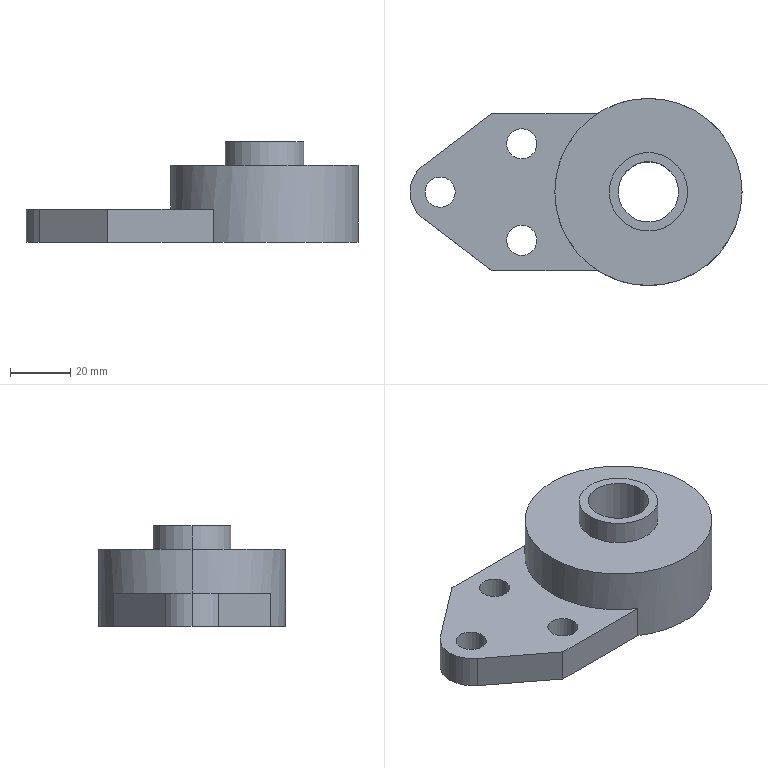Part | SolidWorks | features ICE 2, Extrusion 1 | 1 solid | 22 faces | box 110 x 62 x 33.3 mm | volume 91720 mm3 | cylinder 14 | plane 8 | commonest cylinder face diameters 10 x6 20 x2 22 x2 26 x2 62 x2
STEP:
#1=CARTESIAN_POINT('',(13.,0.,33.3));
#2=VERTEX_POINT('',#1);
#3=CARTESIAN_POINT('',(-13.,0.,33.3));
#4=VERTEX_POINT('',#3);
#5=CARTESIAN_POINT('',(0.,0.,33.3));
#6=DIRECTION('',(0.,0.,1.));
#7=DIRECTION('',(1.,0.,0.));
#8=AXIS2_PLACEMENT_3D('',#5,#6,#7);
#9=CIRCLE('',#8,13.);
#10=EDGE_CURVE('',#2,#4,#9,.T.);
#11=ORIENTED_EDGE('',*,*,#10,.F.);
#12=CARTESIAN_POINT('',(13.,0.,25.5));
#13=VERTEX_POINT('',#12);
#14=CARTESIAN_POINT('',(13.,0.,33.3));
#15=DIRECTION('',(0.,0.,-1.));
#16=VECTOR('',#15,1000.);
#17=LINE('',#14,#16);
#18=EDGE_CURVE('',#2,#13,#17,.T.);
#19=ORIENTED_EDGE('',*,*,#18,.T.);
#20=CARTESIAN_POINT('',(-13.,0.,25.5));
#21=VERTEX_POINT('',#20);
#22=CARTESIAN_POINT('',(0.,0.,25.5));
#23=DIRECTION('',(0.,0.,1.));
#24=DIRECTION('',(1.,0.,0.));
#25=AXIS2_PLACEMENT_3D('',#22,#23,#24);
#26=CIRCLE('',#25,13.);
#27=EDGE_CURVE('',#13,#21,#26,.T.);
#28=ORIENTED_EDGE('',*,*,#27,.T.);
#29=CARTESIAN_POINT('',(-13.,0.,33.3));
#30=DIRECTION('',(0.,0.,-1.));
#31=VECTOR('',#30,1000.);
#32=LINE('',#29,#31);
#33=EDGE_CURVE('',#4,#21,#32,.T.);
#34=ORIENTED_EDGE('',*,*,#33,.F.);
#35=EDGE_LOOP('',(#11,#19,#28,#34));
#36=FACE_OUTER_BOUND('',#35,.T.);
#37=CARTESIAN_POINT('',(0.,0.,33.3));
#38=DIRECTION('',(0.,0.,-1.));
#39=DIRECTION('',(-1.,0.,0.));
#40=AXIS2_PLACEMENT_3D('',#37,#38,#39);
#41=CYLINDRICAL_SURFACE('',#40,13.);
#42=ADVANCED_FACE('',(#36),#41,.T.);
#43=CARTESIAN_POINT('',(-37.,-16.,11.));
#44=VERTEX_POINT('',#43);
#45=CARTESIAN_POINT('',(-47.,-16.,11.));
#46=VERTEX_POINT('',#45);
#47=CARTESIAN_POINT('',(-42.,-16.,11.));
#48=DIRECTION('',(0.,0.,-1.));
#49=DIRECTION('',(-1.,0.,0.));
#50=AXIS2_PLACEMENT_3D('',#47,#48,#49);
#51=CIRCLE('',#50,5.);
#52=EDGE_CURVE('',#44,#46,#51,.T.);
#53=ORIENTED_EDGE('',*,*,#52,.F.);
#54=CARTESIAN_POINT('',(-37.,-16.,0.));
#55=VERTEX_POINT('',#54);
#56=CARTESIAN_POINT('',(-37.,-16.,11.));
#57=DIRECTION('',(0.,0.,-1.));
#58=VECTOR('',#57,1000.);
#59=LINE('',#56,#58);
#60=EDGE_CURVE('',#44,#55,#59,.T.);
#61=ORIENTED_EDGE('',*,*,#60,.T.);
#62=CARTESIAN_POINT('',(-47.,-16.,0.));
#63=VERTEX_POINT('',#62);
#64=CARTESIAN_POINT('',(-42.,-16.,0.));
#65=DIRECTION('',(0.,0.,-1.));
#66=DIRECTION('',(-1.,0.,0.));
#67=AXIS2_PLACEMENT_3D('',#64,#65,#66);
#68=CIRCLE('',#67,5.);
#69=EDGE_CURVE('',#55,#63,#68,.T.);
#70=ORIENTED_EDGE('',*,*,#69,.T.);
#71=CARTESIAN_POINT('',(-47.,-16.,11.));
#72=DIRECTION('',(0.,0.,-1.));
#73=VECTOR('',#72,1000.);
#74=LINE('',#71,#73);
#75=EDGE_CURVE('',#46,#63,#74,.T.);
#76=ORIENTED_EDGE('',*,*,#75,.F.);
#77=EDGE_LOOP('',(#53,#61,#70,#76));
#78=FACE_OUTER_BOUND('',#77,.T.);
#79=CARTESIAN_POINT('',(-42.,-16.,11.));
#80=DIRECTION('',(0.,0.,-1.));
#81=DIRECTION('',(-1.,0.,0.));
#82=AXIS2_PLACEMENT_3D('',#79,#80,#81);
#83=CYLINDRICAL_SURFACE('',#82,5.);
#84=ADVANCED_FACE('',(#78),#83,.F.);
#85=CARTESIAN_POINT('',(-37.,16.,11.));
#86=VERTEX_POINT('',#85);
#87=CARTESIAN_POINT('',(-47.,16.,11.));
#88=VERTEX_POINT('',#87);
#89=CARTESIAN_POINT('',(-42.,16.,11.));
#90=DIRECTION('',(0.,0.,-1.));
#91=DIRECTION('',(-1.,0.,0.));
#92=AXIS2_PLACEMENT_3D('',#89,#90,#91);
#93=CIRCLE('',#92,5.);
#94=EDGE_CURVE('',#86,#88,#93,.T.);
#95=ORIENTED_EDGE('',*,*,#94,.F.);
#96=CARTESIAN_POINT('',(-37.,16.,0.));
#97=VERTEX_POINT('',#96);
#98=CARTESIAN_POINT('',(-37.,16.,11.));
#99=DIRECTION('',(0.,0.,-1.));
#100=VECTOR('',#99,1000.);
#101=LINE('',#98,#100);
#102=EDGE_CURVE('',#86,#97,#101,.T.);
#103=ORIENTED_EDGE('',*,*,#102,.T.);
#104=CARTESIAN_POINT('',(-47.,16.,0.));
#105=VERTEX_POINT('',#104);
#106=CARTESIAN_POINT('',(-42.,16.,0.));
#107=DIRECTION('',(0.,0.,-1.));
#108=DIRECTION('',(-1.,0.,0.));
#109=AXIS2_PLACEMENT_3D('',#106,#107,#108);
#110=CIRCLE('',#109,5.);
#111=EDGE_CURVE('',#97,#105,#110,.T.);
#112=ORIENTED_EDGE('',*,*,#111,.T.);
#113=CARTESIAN_POINT('',(-47.,16.,11.));
#114=DIRECTION('',(0.,0.,-1.));
#115=VECTOR('',#114,1000.);
#116=LINE('',#113,#115);
#117=EDGE_CURVE('',#88,#105,#116,.T.);
#118=ORIENTED_EDGE('',*,*,#117,.F.);
#119=EDGE_LOOP('',(#95,#103,#112,#118));
#120=FACE_OUTER_BOUND('',#119,.T.);
#121=CARTESIAN_POINT('',(-42.,16.,11.));
#122=DIRECTION('',(0.,0.,-1.));
#123=DIRECTION('',(-1.,0.,0.));
#124=AXIS2_PLACEMENT_3D('',#121,#122,#123);
#125=CYLINDRICAL_SURFACE('',#124,5.);
#126=ADVANCED_FACE('',(#120),#125,.F.);
#127=CARTESIAN_POINT('',(-64.,0.,11.));
#128=VERTEX_POINT('',#127);
#129=CARTESIAN_POINT('',(-74.,0.,11.));
#130=VERTEX_POINT('',#129);
#131=CARTESIAN_POINT('',(-69.,0.,11.));
#132=DIRECTION('',(0.,0.,-1.));
#133=DIRECTION('',(-1.,0.,0.));
#134=AXIS2_PLACEMENT_3D('',#131,#132,#133);
#135=CIRCLE('',#134,5.);
#136=EDGE_CURVE('',#128,#130,#135,.T.);
#137=ORIENTED_EDGE('',*,*,#136,.F.);
#138=CARTESIAN_POINT('',(-64.,0.,0.));
#139=VERTEX_POINT('',#138);
#140=CARTESIAN_POINT('',(-64.,0.,11.));
#141=DIRECTION('',(0.,0.,-1.));
#142=VECTOR('',#141,1000.);
#143=LINE('',#140,#142);
#144=EDGE_CURVE('',#128,#139,#143,.T.);
#145=ORIENTED_EDGE('',*,*,#144,.T.);
#146=CARTESIAN_POINT('',(-74.,0.,0.));
#147=VERTEX_POINT('',#146);
#148=CARTESIAN_POINT('',(-69.,0.,0.));
#149=DIRECTION('',(0.,0.,-1.));
#150=DIRECTION('',(-1.,0.,0.));
#151=AXIS2_PLACEMENT_3D('',#148,#149,#150);
#152=CIRCLE('',#151,5.);
#153=EDGE_CURVE('',#139,#147,#152,.T.);
#154=ORIENTED_EDGE('',*,*,#153,.T.);
#155=CARTESIAN_POINT('',(-74.,0.,11.));
#156=DIRECTION('',(0.,0.,-1.));
#157=VECTOR('',#156,1000.);
#158=LINE('',#155,#157);
#159=EDGE_CURVE('',#130,#147,#158,.T.);
#160=ORIENTED_EDGE('',*,*,#159,.F.);
#161=EDGE_LOOP('',(#137,#145,#154,#160));
#162=FACE_OUTER_BOUND('',#161,.T.);
#163=CARTESIAN_POINT('',(-69.,0.,11.));
#164=DIRECTION('',(0.,0.,-1.));
#165=DIRECTION('',(-1.,0.,0.));
#166=AXIS2_PLACEMENT_3D('',#163,#164,#165);
#167=CYLINDRICAL_SURFACE('',#166,5.);
#168=ADVANCED_FACE('',(#162),#167,.F.);
#169=CARTESIAN_POINT('',(-74.662,-8.753,11.));
#170=VERTEX_POINT('',#169);
#171=CARTESIAN_POINT('',(-79.,0.,11.));
#172=VERTEX_POINT('',#171);
#173=CARTESIAN_POINT('',(-68.,0.,11.));
#174=DIRECTION('',(0.,0.,-1.));
#175=DIRECTION('',(-1.,0.,0.));
#176=AXIS2_PLACEMENT_3D('',#173,#174,#175);
#177=CIRCLE('',#176,11.);
#178=EDGE_CURVE('',#170,#172,#177,.T.);
#179=ORIENTED_EDGE('',*,*,#178,.T.);
#180=CARTESIAN_POINT('',(-79.,0.,0.));
#181=VERTEX_POINT('',#180);
#182=CARTESIAN_POINT('',(-79.,0.,11.));
#183=DIRECTION('',(0.,0.,-1.));
#184=VECTOR('',#183,1000.);
#185=LINE('',#182,#184);
#186=EDGE_CURVE('',#172,#181,#185,.T.);
#187=ORIENTED_EDGE('',*,*,#186,.T.);
#188=CARTESIAN_POINT('',(-74.662,-8.753,0.));
#189=VERTEX_POINT('',#188);
#190=CARTESIAN_POINT('',(-68.,0.,0.));
#191=DIRECTION('',(0.,0.,-1.));
#192=DIRECTION('',(-1.,0.,0.));
#193=AXIS2_PLACEMENT_3D('',#190,#191,#192);
#194=CIRCLE('',#193,11.);
#195=EDGE_CURVE('',#189,#181,#194,.T.);
#196=ORIENTED_EDGE('',*,*,#195,.F.);
#197=CARTESIAN_POINT('',(-74.662,-8.753,11.));
#198=DIRECTION('',(0.,0.,-1.));
#199=VECTOR('',#198,1000.);
#200=LINE('',#197,#199);
#201=EDGE_CURVE('',#170,#189,#200,.T.);
#202=ORIENTED_EDGE('',*,*,#201,.F.);
#203=EDGE_LOOP('',(#179,#187,#196,#202));
#204=FACE_OUTER_BOUND('',#203,.T.);
#205=CARTESIAN_POINT('',(-68.,0.,11.));
#206=DIRECTION('',(0.,0.,-1.));
#207=DIRECTION('',(-1.,0.,0.));
#208=AXIS2_PLACEMENT_3D('',#205,#206,#207);
#209=CYLINDRICAL_SURFACE('',#208,11.);
#210=ADVANCED_FACE('',(#204),#209,.T.);
#211=CARTESIAN_POINT('',(-10.,0.,33.3));
#212=VERTEX_POINT('',#211);
#213=CARTESIAN_POINT('',(10.,0.,33.3));
#214=VERTEX_POINT('',#213);
#215=CARTESIAN_POINT('',(0.,0.,33.3));
#216=DIRECTION('',(0.,0.,1.));
#217=DIRECTION('',(1.,0.,0.));
#218=AXIS2_PLACEMENT_3D('',#215,#216,#217);
#219=CIRCLE('',#218,10.);
#220=EDGE_CURVE('',#212,#214,#219,.T.);
#221=ORIENTED_EDGE('',*,*,#220,.T.);
#222=CARTESIAN_POINT('',(10.,0.,0.));
#223=VERTEX_POINT('',#222);
#224=CARTESIAN_POINT('',(10.,0.,25.5));
#225=DIRECTION('',(0.,0.,-1.));
#226=VECTOR('',#225,1000.);
#227=LINE('',#224,#226);
#228=EDGE_CURVE('',#214,#223,#227,.T.);
#229=ORIENTED_EDGE('',*,*,#228,.T.);
#230=CARTESIAN_POINT('',(-10.,0.,0.));
#231=VERTEX_POINT('',#230);
#232=CARTESIAN_POINT('',(0.,0.,0.));
#233=DIRECTION('',(0.,0.,1.));
#234=DIRECTION('',(1.,0.,0.));
#235=AXIS2_PLACEMENT_3D('',#232,#233,#234);
#236=CIRCLE('',#235,10.);
#237=EDGE_CURVE('',#231,#223,#236,.T.);
#238=ORIENTED_EDGE('',*,*,#237,.F.);
#239=CARTESIAN_POINT('',(-10.,0.,25.5));
#240=DIRECTION('',(0.,0.,-1.));
#241=VECTOR('',#240,1000.);
#242=LINE('',#239,#241);
#243=EDGE_CURVE('',#212,#231,#242,.T.);
#244=ORIENTED_EDGE('',*,*,#243,.F.);
#245=EDGE_LOOP('',(#221,#229,#238,#244));
#246=FACE_OUTER_BOUND('',#245,.T.);
#247=CARTESIAN_POINT('',(0.,0.,25.5));
#248=DIRECTION('',(0.,0.,-1.));
#249=DIRECTION('',(-1.,0.,0.));
#250=AXIS2_PLACEMENT_3D('',#247,#248,#249);
#251=CYLINDRICAL_SURFACE('',#250,10.);
#252=ADVANCED_FACE('',(#246),#251,.F.);
#253=CARTESIAN_POINT('',(31.,0.,25.5));
#254=VERTEX_POINT('',#253);
#255=CARTESIAN_POINT('',(-31.,0.,25.5));
#256=VERTEX_POINT('',#255);
#257=CARTESIAN_POINT('',(0.,0.,25.5));
#258=DIRECTION('',(0.,0.,1.));
#259=DIRECTION('',(1.,0.,0.));
#260=AXIS2_PLACEMENT_3D('',#257,#258,#259);
#261=CIRCLE('',#260,31.);
#262=EDGE_CURVE('',#254,#256,#261,.T.);
#263=ORIENTED_EDGE('',*,*,#262,.F.);
#264=CARTESIAN_POINT('',(31.,0.,0.));
#265=VERTEX_POINT('',#264);
#266=CARTESIAN_POINT('',(31.,0.,25.5));
#267=DIRECTION('',(0.,0.,-1.));
#268=VECTOR('',#267,1000.);
#269=LINE('',#266,#268);
#270=EDGE_CURVE('',#254,#265,#269,.T.);
#271=ORIENTED_EDGE('',*,*,#270,.T.);
#272=CARTESIAN_POINT('',(-16.882,26.,0.));
#273=VERTEX_POINT('',#272);
#274=CARTESIAN_POINT('',(0.,0.,0.));
#275=DIRECTION('',(0.,0.,1.));
#276=DIRECTION('',(1.,0.,0.));
#277=AXIS2_PLACEMENT_3D('',#274,#275,#276);
#278=CIRCLE('',#277,31.);
#279=EDGE_CURVE('',#265,#273,#278,.T.);
#280=ORIENTED_EDGE('',*,*,#279,.T.);
#281=CARTESIAN_POINT('',(-16.882,26.,11.));
#282=VERTEX_POINT('',#281);
#283=CARTESIAN_POINT('',(-16.882,26.,11.));
#284=DIRECTION('',(0.,0.,-1.));
#285=VECTOR('',#284,1000.);
#286=LINE('',#283,#285);
#287=EDGE_CURVE('',#282,#273,#286,.T.);
#288=ORIENTED_EDGE('',*,*,#287,.F.);
#289=CARTESIAN_POINT('',(-31.,0.,11.));
#290=VERTEX_POINT('',#289);
#291=CARTESIAN_POINT('',(0.,0.,11.));
#292=DIRECTION('',(0.,0.,1.));
#293=DIRECTION('',(-1.,0.,0.));
#294=AXIS2_PLACEMENT_3D('',#291,#292,#293);
#295=CIRCLE('',#294,31.);
#296=EDGE_CURVE('',#282,#290,#295,.T.);
#297=ORIENTED_EDGE('',*,*,#296,.T.);
#298=CARTESIAN_POINT('',(-31.,0.,25.5));
#299=DIRECTION('',(0.,0.,-1.));
#300=VECTOR('',#299,1000.);
#301=LINE('',#298,#300);
#302=EDGE_CURVE('',#256,#290,#301,.T.);
#303=ORIENTED_EDGE('',*,*,#302,.F.);
#304=EDGE_LOOP('',(#263,#271,#280,#288,#297,#303));
#305=FACE_OUTER_BOUND('',#304,.T.);
#306=CARTESIAN_POINT('',(0.,0.,25.5));
#307=DIRECTION('',(0.,0.,-1.));
#308=DIRECTION('',(-1.,0.,0.));
#309=AXIS2_PLACEMENT_3D('',#306,#307,#308);
#310=CYLINDRICAL_SURFACE('',#309,31.);
#311=ADVANCED_FACE('',(#305),#310,.T.);
#312=CARTESIAN_POINT('',(0.,0.,25.5));
#313=DIRECTION('',(0.,0.,1.));
#314=DIRECTION('',(1.,0.,0.));
#315=AXIS2_PLACEMENT_3D('',#312,#313,#314);
#316=CIRCLE('',#315,31.);
#317=EDGE_CURVE('',#256,#254,#316,.T.);
#318=ORIENTED_EDGE('',*,*,#317,.T.);
#319=ORIENTED_EDGE('',*,*,#262,.T.);
#320=EDGE_LOOP('',(#318,#319));
#321=FACE_OUTER_BOUND('',#320,.T.);
#322=CARTESIAN_POINT('',(0.,0.,25.5));
#323=DIRECTION('',(0.,0.,1.));
#324=DIRECTION('',(1.,0.,0.));
#325=AXIS2_PLACEMENT_3D('',#322,#323,#324);
#326=CIRCLE('',#325,13.);
#327=EDGE_CURVE('',#21,#13,#326,.T.);
#328=ORIENTED_EDGE('',*,*,#327,.F.);
#329=ORIENTED_EDGE('',*,*,#27,.F.);
#330=EDGE_LOOP('',(#328,#329));
#331=FACE_BOUND('',#330,.T.);
#332=CARTESIAN_POINT('',(0.,0.,25.5));
#333=DIRECTION('',(0.,0.,1.));
#334=DIRECTION('',(1.,0.,0.));
#335=AXIS2_PLACEMENT_3D('',#332,#333,#334);
#336=PLANE('',#335);
#337=ADVANCED_FACE('',(#321,#331),#336,.T.);
#338=CARTESIAN_POINT('',(-16.882,-26.,0.));
#339=VERTEX_POINT('',#338);
#340=CARTESIAN_POINT('',(0.,0.,0.));
#341=DIRECTION('',(0.,0.,1.));
#342=DIRECTION('',(1.,0.,0.));
#343=AXIS2_PLACEMENT_3D('',#340,#341,#342);
#344=CIRCLE('',#343,31.);
#345=EDGE_CURVE('',#339,#265,#344,.T.);
#346=ORIENTED_EDGE('',*,*,#345,.F.);
#347=CARTESIAN_POINT('',(-52.,-26.,0.));
#348=VERTEX_POINT('',#347);
#349=CARTESIAN_POINT('',(-16.882,-26.,0.));
#350=DIRECTION('',(-1.,0.,0.));
#351=VECTOR('',#350,1000.);
#352=LINE('',#349,#351);
#353=EDGE_CURVE('',#339,#348,#352,.T.);
#354=ORIENTED_EDGE('',*,*,#353,.T.);
#355=CARTESIAN_POINT('',(-52.,-26.,0.));
#356=DIRECTION('',(-0.7958,0.6056,0.));
#357=VECTOR('',#356,1000.);
#358=LINE('',#355,#357);
#359=EDGE_CURVE('',#348,#189,#358,.T.);
#360=ORIENTED_EDGE('',*,*,#359,.T.);
#361=ORIENTED_EDGE('',*,*,#195,.T.);
#362=CARTESIAN_POINT('',(-74.662,8.753,0.));
#363=VERTEX_POINT('',#362);
#364=CARTESIAN_POINT('',(-68.,0.,0.));
#365=DIRECTION('',(0.,0.,-1.));
#366=DIRECTION('',(-1.,0.,0.));
#367=AXIS2_PLACEMENT_3D('',#364,#365,#366);
#368=CIRCLE('',#367,11.);
#369=EDGE_CURVE('',#181,#363,#368,.T.);
#370=ORIENTED_EDGE('',*,*,#369,.T.);
#371=CARTESIAN_POINT('',(-52.,26.,0.));
#372=VERTEX_POINT('',#371);
#373=CARTESIAN_POINT('',(-52.,26.,0.));
#374=DIRECTION('',(0.7958,0.6056,0.));
#375=VECTOR('',#374,1000.);
#376=LINE('',#373,#375);
#377=EDGE_CURVE('',#363,#372,#376,.T.);
#378=ORIENTED_EDGE('',*,*,#377,.T.);
#379=CARTESIAN_POINT('',(-16.882,26.,0.));
#380=DIRECTION('',(1.,0.,0.));
#381=VECTOR('',#380,1000.);
#382=LINE('',#379,#381);
#383=EDGE_CURVE('',#372,#273,#382,.T.);
#384=ORIENTED_EDGE('',*,*,#383,.T.);
#385=ORIENTED_EDGE('',*,*,#279,.F.);
#386=EDGE_LOOP('',(#346,#354,#360,#361,#370,#378,#384,#385));
#387=FACE_OUTER_BOUND('',#386,.T.);
#388=ORIENTED_EDGE('',*,*,#237,.T.);
#389=CARTESIAN_POINT('',(0.,0.,0.));
#390=DIRECTION('',(0.,0.,1.));
#391=DIRECTION('',(1.,0.,0.));
#392=AXIS2_PLACEMENT_3D('',#389,#390,#391);
#393=CIRCLE('',#392,10.);
#394=EDGE_CURVE('',#223,#231,#393,.T.);
#395=ORIENTED_EDGE('',*,*,#394,.T.);
#396=EDGE_LOOP('',(#388,#395));
#397=FACE_BOUND('',#396,.T.);
#398=CARTESIAN_POINT('',(-42.,-16.,0.));
#399=DIRECTION('',(0.,0.,-1.));
#400=DIRECTION('',(-1.,0.,0.));
#401=AXIS2_PLACEMENT_3D('',#398,#399,#400);
#402=CIRCLE('',#401,5.);
#403=EDGE_CURVE('',#63,#55,#402,.T.);
#404=ORIENTED_EDGE('',*,*,#403,.F.);
#405=ORIENTED_EDGE('',*,*,#69,.F.);
#406=EDGE_LOOP('',(#404,#405));
#407=FACE_BOUND('',#406,.T.);
#408=CARTESIAN_POINT('',(-42.,16.,0.));
#409=DIRECTION('',(0.,0.,-1.));
#410=DIRECTION('',(-1.,0.,0.));
#411=AXIS2_PLACEMENT_3D('',#408,#409,#410);
#412=CIRCLE('',#411,5.);
#413=EDGE_CURVE('',#105,#97,#412,.T.);
#414=ORIENTED_EDGE('',*,*,#413,.F.);
#415=ORIENTED_EDGE('',*,*,#111,.F.);
#416=EDGE_LOOP('',(#414,#415));
#417=FACE_BOUND('',#416,.T.);
#418=CARTESIAN_POINT('',(-69.,0.,0.));
#419=DIRECTION('',(0.,0.,-1.));
#420=DIRECTION('',(-1.,0.,0.));
#421=AXIS2_PLACEMENT_3D('',#418,#419,#420);
#422=CIRCLE('',#421,5.);
#423=EDGE_CURVE('',#147,#139,#422,.T.);
#424=ORIENTED_EDGE('',*,*,#423,.F.);
#425=ORIENTED_EDGE('',*,*,#153,.F.);
#426=EDGE_LOOP('',(#424,#425));
#427=FACE_BOUND('',#426,.T.);
#428=CARTESIAN_POINT('',(0.,0.,0.));
#429=DIRECTION('',(0.,0.,1.));
#430=DIRECTION('',(1.,0.,0.));
#431=AXIS2_PLACEMENT_3D('',#428,#429,#430);
#432=PLANE('',#431);
#433=ADVANCED_FACE('',(#387,#397,#407,#417,#427),#432,.F.);
#434=ORIENTED_EDGE('',*,*,#270,.F.);
#435=ORIENTED_EDGE('',*,*,#317,.F.);
#436=ORIENTED_EDGE('',*,*,#302,.T.);
#437=CARTESIAN_POINT('',(-16.882,-26.,11.));
#438=VERTEX_POINT('',#437);
#439=CARTESIAN_POINT('',(0.,0.,11.));
#440=DIRECTION('',(0.,0.,1.));
#441=DIRECTION('',(-1.,0.,0.));
#442=AXIS2_PLACEMENT_3D('',#439,#440,#441);
#443=CIRCLE('',#442,31.);
#444=EDGE_CURVE('',#290,#438,#443,.T.);
#445=ORIENTED_EDGE('',*,*,#444,.T.);
#446=CARTESIAN_POINT('',(-16.882,-26.,11.));
#447=DIRECTION('',(0.,0.,-1.));
#448=VECTOR('',#447,1000.);
#449=LINE('',#446,#448);
#450=EDGE_CURVE('',#438,#339,#449,.T.);
#451=ORIENTED_EDGE('',*,*,#450,.T.);
#452=ORIENTED_EDGE('',*,*,#345,.T.);
#453=EDGE_LOOP('',(#434,#435,#436,#445,#451,#452));
#454=FACE_OUTER_BOUND('',#453,.T.);
#455=CARTESIAN_POINT('',(0.,0.,25.5));
#456=DIRECTION('',(0.,0.,-1.));
#457=DIRECTION('',(-1.,0.,0.));
#458=AXIS2_PLACEMENT_3D('',#455,#456,#457);
#459=CYLINDRICAL_SURFACE('',#458,31.);
#460=ADVANCED_FACE('',(#454),#459,.T.);
#461=ORIENTED_EDGE('',*,*,#228,.F.);
#462=CARTESIAN_POINT('',(0.,0.,33.3));
#463=DIRECTION('',(0.,0.,1.));
#464=DIRECTION('',(1.,0.,0.));
#465=AXIS2_PLACEMENT_3D('',#462,#463,#464);
#466=CIRCLE('',#465,10.);
#467=EDGE_CURVE('',#214,#212,#466,.T.);
#468=ORIENTED_EDGE('',*,*,#467,.T.);
#469=ORIENTED_EDGE('',*,*,#243,.T.);
#470=ORIENTED_EDGE('',*,*,#394,.F.);
#471=EDGE_LOOP('',(#461,#468,#469,#470));
#472=FACE_OUTER_BOUND('',#471,.T.);
#473=CARTESIAN_POINT('',(0.,0.,25.5));
#474=DIRECTION('',(0.,0.,-1.));
#475=DIRECTION('',(-1.,0.,0.));
#476=AXIS2_PLACEMENT_3D('',#473,#474,#475);
#477=CYLINDRICAL_SURFACE('',#476,10.);
#478=ADVANCED_FACE('',(#472),#477,.F.);
#479=ORIENTED_EDGE('',*,*,#377,.F.);
#480=CARTESIAN_POINT('',(-74.662,8.753,11.));
#481=VERTEX_POINT('',#480);
#482=CARTESIAN_POINT('',(-74.662,8.753,11.));
#483=DIRECTION('',(0.,0.,-1.));
#484=VECTOR('',#483,1000.);
#485=LINE('',#482,#484);
#486=EDGE_CURVE('',#481,#363,#485,.T.);
#487=ORIENTED_EDGE('',*,*,#486,.F.);
#488=CARTESIAN_POINT('',(-52.,26.,11.));
#489=VERTEX_POINT('',#488);
#490=CARTESIAN_POINT('',(-52.,26.,11.));
#491=DIRECTION('',(0.7958,0.6056,0.));
#492=VECTOR('',#491,1000.);
#493=LINE('',#490,#492);
#494=EDGE_CURVE('',#481,#489,#493,.T.);
#495=ORIENTED_EDGE('',*,*,#494,.T.);
#496=CARTESIAN_POINT('',(-52.,26.,11.));
#497=DIRECTION('',(0.,0.,-1.));
#498=VECTOR('',#497,1000.);
#499=LINE('',#496,#498);
#500=EDGE_CURVE('',#489,#372,#499,.T.);
#501=ORIENTED_EDGE('',*,*,#500,.T.);
#502=EDGE_LOOP('',(#479,#487,#495,#501));
#503=FACE_OUTER_BOUND('',#502,.T.);
#504=CARTESIAN_POINT('',(-52.,26.,11.));
#505=DIRECTION('',(-0.6056,0.7958,0.));
#506=DIRECTION('',(-0.7958,-0.6056,0.));
#507=AXIS2_PLACEMENT_3D('',#504,#505,#506);
#508=PLANE('',#507);
#509=ADVANCED_FACE('',(#503),#508,.T.);
#510=ORIENTED_EDGE('',*,*,#186,.F.);
#511=CARTESIAN_POINT('',(-68.,0.,11.));
#512=DIRECTION('',(0.,0.,-1.));
#513=DIRECTION('',(-1.,0.,0.));
#514=AXIS2_PLACEMENT_3D('',#511,#512,#513);
#515=CIRCLE('',#514,11.);
#516=EDGE_CURVE('',#172,#481,#515,.T.);
#517=ORIENTED_EDGE('',*,*,#516,.T.);
#518=ORIENTED_EDGE('',*,*,#486,.T.);
#519=ORIENTED_EDGE('',*,*,#369,.F.);
#520=EDGE_LOOP('',(#510,#517,#518,#519));
#521=FACE_OUTER_BOUND('',#520,.T.);
#522=CARTESIAN_POINT('',(-68.,0.,11.));
#523=DIRECTION('',(0.,0.,-1.));
#524=DIRECTION('',(-1.,0.,0.));
#525=AXIS2_PLACEMENT_3D('',#522,#523,#524);
#526=CYLINDRICAL_SURFACE('',#525,11.);
#527=ADVANCED_FACE('',(#521),#526,.T.);
#528=ORIENTED_EDGE('',*,*,#359,.F.);
#529=CARTESIAN_POINT('',(-52.,-26.,11.));
#530=VERTEX_POINT('',#529);
#531=CARTESIAN_POINT('',(-52.,-26.,11.));
#532=DIRECTION('',(0.,0.,-1.));
#533=VECTOR('',#532,1000.);
#534=LINE('',#531,#533);
#535=EDGE_CURVE('',#530,#348,#534,.T.);
#536=ORIENTED_EDGE('',*,*,#535,.F.);
#537=CARTESIAN_POINT('',(-52.,-26.,11.));
#538=DIRECTION('',(-0.7958,0.6056,0.));
#539=VECTOR('',#538,1000.);
#540=LINE('',#537,#539);
#541=EDGE_CURVE('',#530,#170,#540,.T.);
#542=ORIENTED_EDGE('',*,*,#541,.T.);
#543=ORIENTED_EDGE('',*,*,#201,.T.);
#544=EDGE_LOOP('',(#528,#536,#542,#543));
#545=FACE_OUTER_BOUND('',#544,.T.);
#546=CARTESIAN_POINT('',(-52.,-26.,11.));
#547=DIRECTION('',(-0.6056,-0.7958,0.));
#548=DIRECTION('',(0.7958,-0.6056,0.));
#549=AXIS2_PLACEMENT_3D('',#546,#547,#548);
#550=PLANE('',#549);
#551=ADVANCED_FACE('',(#545),#550,.T.);
#552=ORIENTED_EDGE('',*,*,#353,.F.);
#553=ORIENTED_EDGE('',*,*,#450,.F.);
#554=CARTESIAN_POINT('',(-16.882,-26.,11.));
#555=DIRECTION('',(-1.,0.,0.));
#556=VECTOR('',#555,1000.);
#557=LINE('',#554,#556);
#558=EDGE_CURVE('',#438,#530,#557,.T.);
#559=ORIENTED_EDGE('',*,*,#558,.T.);
#560=ORIENTED_EDGE('',*,*,#535,.T.);
#561=EDGE_LOOP('',(#552,#553,#559,#560));
#562=FACE_OUTER_BOUND('',#561,.T.);
#563=CARTESIAN_POINT('',(-16.882,-26.,11.));
#564=DIRECTION('',(0.,-1.,0.));
#565=DIRECTION('',(1.,0.,0.));
#566=AXIS2_PLACEMENT_3D('',#563,#564,#565);
#567=PLANE('',#566);
#568=ADVANCED_FACE('',(#562),#567,.T.);
#569=ORIENTED_EDGE('',*,*,#383,.F.);
#570=ORIENTED_EDGE('',*,*,#500,.F.);
#571=CARTESIAN_POINT('',(-16.882,26.,11.));
#572=DIRECTION('',(1.,0.,0.));
#573=VECTOR('',#572,1000.);
#574=LINE('',#571,#573);
#575=EDGE_CURVE('',#489,#282,#574,.T.);
#576=ORIENTED_EDGE('',*,*,#575,.T.);
#577=ORIENTED_EDGE('',*,*,#287,.T.);
#578=EDGE_LOOP('',(#569,#570,#576,#577));
#579=FACE_OUTER_BOUND('',#578,.T.);
#580=CARTESIAN_POINT('',(-16.882,26.,11.));
#581=DIRECTION('',(0.,1.,0.));
#582=DIRECTION('',(-1.,0.,0.));
#583=AXIS2_PLACEMENT_3D('',#580,#581,#582);
#584=PLANE('',#583);
#585=ADVANCED_FACE('',(#579),#584,.T.);
#586=CARTESIAN_POINT('',(-42.,-16.,11.));
#587=DIRECTION('',(0.,0.,-1.));
#588=DIRECTION('',(-1.,0.,0.));
#589=AXIS2_PLACEMENT_3D('',#586,#587,#588);
#590=CIRCLE('',#589,5.);
#591=EDGE_CURVE('',#46,#44,#590,.T.);
#592=ORIENTED_EDGE('',*,*,#591,.T.);
#593=ORIENTED_EDGE('',*,*,#52,.T.);
#594=EDGE_LOOP('',(#592,#593));
#595=FACE_BOUND('',#594,.T.);
#596=CARTESIAN_POINT('',(-42.,16.,11.));
#597=DIRECTION('',(0.,0.,-1.));
#598=DIRECTION('',(-1.,0.,0.));
#599=AXIS2_PLACEMENT_3D('',#596,#597,#598);
#600=CIRCLE('',#599,5.);
#601=EDGE_CURVE('',#88,#86,#600,.T.);
#602=ORIENTED_EDGE('',*,*,#601,.T.);
#603=ORIENTED_EDGE('',*,*,#94,.T.);
#604=EDGE_LOOP('',(#602,#603));
#605=FACE_BOUND('',#604,.T.);
#606=CARTESIAN_POINT('',(-69.,0.,11.));
#607=DIRECTION('',(0.,0.,-1.));
#608=DIRECTION('',(-1.,0.,0.));
#609=AXIS2_PLACEMENT_3D('',#606,#607,#608);
#610=CIRCLE('',#609,5.);
#611=EDGE_CURVE('',#130,#128,#610,.T.);
#612=ORIENTED_EDGE('',*,*,#611,.T.);
#613=ORIENTED_EDGE('',*,*,#136,.T.);
#614=EDGE_LOOP('',(#612,#613));
#615=FACE_BOUND('',#614,.T.);
#616=ORIENTED_EDGE('',*,*,#494,.F.);
#617=ORIENTED_EDGE('',*,*,#516,.F.);
#618=ORIENTED_EDGE('',*,*,#178,.F.);
#619=ORIENTED_EDGE('',*,*,#541,.F.);
#620=ORIENTED_EDGE('',*,*,#558,.F.);
#621=ORIENTED_EDGE('',*,*,#444,.F.);
#622=ORIENTED_EDGE('',*,*,#296,.F.);
#623=ORIENTED_EDGE('',*,*,#575,.F.);
#624=EDGE_LOOP('',(#616,#617,#618,#619,#620,#621,#622,#623));
#625=FACE_OUTER_BOUND('',#624,.T.);
#626=CARTESIAN_POINT('',(-68.,0.,11.));
#627=DIRECTION('',(0.,0.,-1.));
#628=DIRECTION('',(-1.,0.,0.));
#629=AXIS2_PLACEMENT_3D('',#626,#627,#628);
#630=PLANE('',#629);
#631=ADVANCED_FACE('',(#595,#605,#615,#625),#630,.F.);
#632=ORIENTED_EDGE('',*,*,#144,.F.);
#633=ORIENTED_EDGE('',*,*,#611,.F.);
#634=ORIENTED_EDGE('',*,*,#159,.T.);
#635=ORIENTED_EDGE('',*,*,#423,.T.);
#636=EDGE_LOOP('',(#632,#633,#634,#635));
#637=FACE_OUTER_BOUND('',#636,.T.);
#638=CARTESIAN_POINT('',(-69.,0.,11.));
#639=DIRECTION('',(0.,0.,-1.));
#640=DIRECTION('',(-1.,0.,0.));
#641=AXIS2_PLACEMENT_3D('',#638,#639,#640);
#642=CYLINDRICAL_SURFACE('',#641,5.);
#643=ADVANCED_FACE('',(#637),#642,.F.);
#644=ORIENTED_EDGE('',*,*,#102,.F.);
#645=ORIENTED_EDGE('',*,*,#601,.F.);
#646=ORIENTED_EDGE('',*,*,#117,.T.);
#647=ORIENTED_EDGE('',*,*,#413,.T.);
#648=EDGE_LOOP('',(#644,#645,#646,#647));
#649=FACE_OUTER_BOUND('',#648,.T.);
#650=CARTESIAN_POINT('',(-42.,16.,11.));
#651=DIRECTION('',(0.,0.,-1.));
#652=DIRECTION('',(-1.,0.,0.));
#653=AXIS2_PLACEMENT_3D('',#650,#651,#652);
#654=CYLINDRICAL_SURFACE('',#653,5.);
#655=ADVANCED_FACE('',(#649),#654,.F.);
#656=ORIENTED_EDGE('',*,*,#60,.F.);
#657=ORIENTED_EDGE('',*,*,#591,.F.);
#658=ORIENTED_EDGE('',*,*,#75,.T.);
#659=ORIENTED_EDGE('',*,*,#403,.T.);
#660=EDGE_LOOP('',(#656,#657,#658,#659));
#661=FACE_OUTER_BOUND('',#660,.T.);
#662=CARTESIAN_POINT('',(-42.,-16.,11.));
#663=DIRECTION('',(0.,0.,-1.));
#664=DIRECTION('',(-1.,0.,0.));
#665=AXIS2_PLACEMENT_3D('',#662,#663,#664);
#666=CYLINDRICAL_SURFACE('',#665,5.);
#667=ADVANCED_FACE('',(#661),#666,.F.);
#668=CARTESIAN_POINT('',(0.,0.,33.3));
#669=DIRECTION('',(0.,0.,1.));
#670=DIRECTION('',(1.,0.,0.));
#671=AXIS2_PLACEMENT_3D('',#668,#669,#670);
#672=CIRCLE('',#671,13.);
#673=EDGE_CURVE('',#4,#2,#672,.T.);
#674=ORIENTED_EDGE('',*,*,#673,.T.);
#675=ORIENTED_EDGE('',*,*,#10,.T.);
#676=EDGE_LOOP('',(#674,#675));
#677=FACE_OUTER_BOUND('',#676,.T.);
#678=ORIENTED_EDGE('',*,*,#220,.F.);
#679=ORIENTED_EDGE('',*,*,#467,.F.);
#680=EDGE_LOOP('',(#678,#679));
#681=FACE_BOUND('',#680,.T.);
#682=CARTESIAN_POINT('',(0.,0.,33.3));
#683=DIRECTION('',(0.,0.,1.));
#684=DIRECTION('',(1.,0.,0.));
#685=AXIS2_PLACEMENT_3D('',#682,#683,#684);
#686=PLANE('',#685);
#687=ADVANCED_FACE('',(#677,#681),#686,.T.);
#688=ORIENTED_EDGE('',*,*,#18,.F.);
#689=ORIENTED_EDGE('',*,*,#673,.F.);
#690=ORIENTED_EDGE('',*,*,#33,.T.);
#691=ORIENTED_EDGE('',*,*,#327,.T.);
#692=EDGE_LOOP('',(#688,#689,#690,#691));
#693=FACE_OUTER_BOUND('',#692,.T.);
#694=CARTESIAN_POINT('',(0.,0.,33.3));
#695=DIRECTION('',(0.,0.,-1.));
#696=DIRECTION('',(-1.,0.,0.));
#697=AXIS2_PLACEMENT_3D('',#694,#695,#696);
#698=CYLINDRICAL_SURFACE('',#697,13.);
#699=ADVANCED_FACE('',(#693),#698,.T.);
#700=CLOSED_SHELL('',(#42,#84,#126,#168,#210,#252,#311,#337,#433,#460,#478,#509,#527,#551,#568,#585,#631,#643,#655,#667,#687,#699));
#701=MANIFOLD_SOLID_BREP('',#700);
#702=CARTESIAN_POINT('',(0.,0.,0.));
#703=DIRECTION('',(0.,0.,1.));
#704=DIRECTION('',(1.,0.,0.));
#705=AXIS2_PLACEMENT_3D('',#702,#703,#704);
#706=(LENGTH_UNIT()NAMED_UNIT(*)SI_UNIT(.MILLI.,.METRE.));
#707=UNCERTAINTY_MEASURE_WITH_UNIT(LENGTH_MEASURE(0.00001),#706,'','');
#708=(NAMED_UNIT(*)PLANE_ANGLE_UNIT()SI_UNIT($,.RADIAN.));
#709=(NAMED_UNIT(*)SI_UNIT($,.STERADIAN.)SOLID_ANGLE_UNIT());
#710=(GEOMETRIC_REPRESENTATION_CONTEXT(3)GLOBAL_UNCERTAINTY_ASSIGNED_CONTEXT((#707))GLOBAL_UNIT_ASSIGNED_CONTEXT((#706,#708,#709))REPRESENTATION_CONTEXT('',''));
#711=ADVANCED_BREP_SHAPE_REPRESENTATION('',(#701,#705),#710);